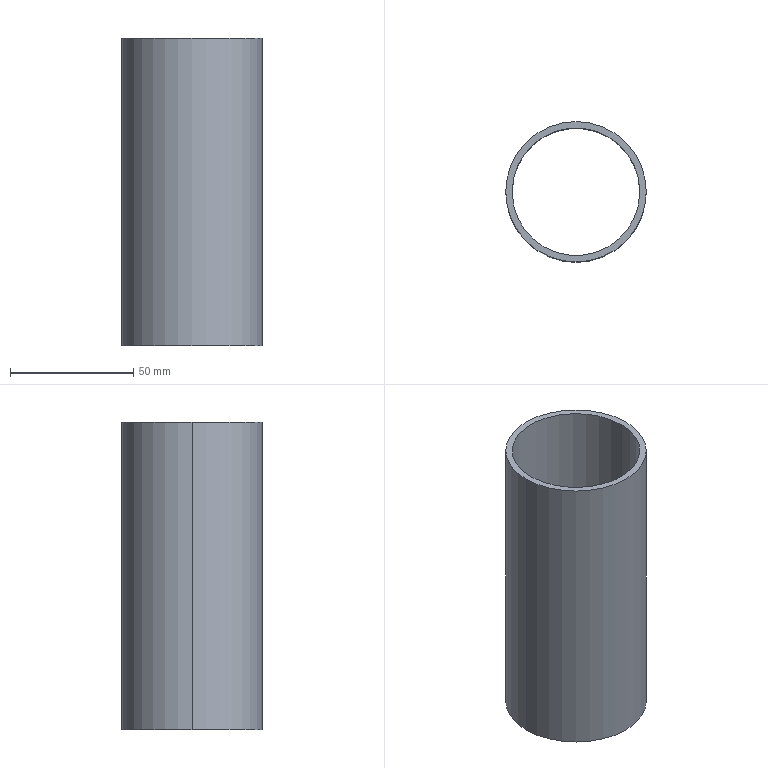Part | SolidWorks | features ExtruThin 1 | 1 solid | 6 faces | box 57 x 57 x 124.7 mm | volume 55410 mm3 | cylinder 4 | plane 2 | commonest cylinder face diameters 51.8 x2 57 x2
STEP:
#1=CARTESIAN_POINT('',(-25.9,0.,124.7));
#2=VERTEX_POINT('',#1);
#3=CARTESIAN_POINT('',(25.9,0.,124.7));
#4=VERTEX_POINT('',#3);
#5=CARTESIAN_POINT('',(0.,0.,124.7));
#6=DIRECTION('',(0.,0.,1.));
#7=DIRECTION('',(1.,0.,0.));
#8=AXIS2_PLACEMENT_3D('',#5,#6,#7);
#9=CIRCLE('',#8,25.9);
#10=EDGE_CURVE('',#2,#4,#9,.T.);
#11=ORIENTED_EDGE('',*,*,#10,.T.);
#12=CARTESIAN_POINT('',(25.9,0.,0.));
#13=VERTEX_POINT('',#12);
#14=CARTESIAN_POINT('',(25.9,0.,124.7));
#15=DIRECTION('',(0.,0.,-1.));
#16=VECTOR('',#15,1000.);
#17=LINE('',#14,#16);
#18=EDGE_CURVE('',#4,#13,#17,.T.);
#19=ORIENTED_EDGE('',*,*,#18,.T.);
#20=CARTESIAN_POINT('',(-25.9,0.,0.));
#21=VERTEX_POINT('',#20);
#22=CARTESIAN_POINT('',(0.,0.,0.));
#23=DIRECTION('',(0.,0.,1.));
#24=DIRECTION('',(1.,0.,0.));
#25=AXIS2_PLACEMENT_3D('',#22,#23,#24);
#26=CIRCLE('',#25,25.9);
#27=EDGE_CURVE('',#21,#13,#26,.T.);
#28=ORIENTED_EDGE('',*,*,#27,.F.);
#29=CARTESIAN_POINT('',(-25.9,0.,124.7));
#30=DIRECTION('',(0.,0.,-1.));
#31=VECTOR('',#30,1000.);
#32=LINE('',#29,#31);
#33=EDGE_CURVE('',#2,#21,#32,.T.);
#34=ORIENTED_EDGE('',*,*,#33,.F.);
#35=EDGE_LOOP('',(#11,#19,#28,#34));
#36=FACE_OUTER_BOUND('',#35,.T.);
#37=CARTESIAN_POINT('',(0.,0.,124.7));
#38=DIRECTION('',(0.,0.,-1.));
#39=DIRECTION('',(-1.,0.,0.));
#40=AXIS2_PLACEMENT_3D('',#37,#38,#39);
#41=CYLINDRICAL_SURFACE('',#40,25.9);
#42=ADVANCED_FACE('',(#36),#41,.F.);
#43=CARTESIAN_POINT('',(28.5,0.,124.7));
#44=VERTEX_POINT('',#43);
#45=CARTESIAN_POINT('',(-28.5,0.,124.7));
#46=VERTEX_POINT('',#45);
#47=CARTESIAN_POINT('',(0.,0.,124.7));
#48=DIRECTION('',(0.,0.,1.));
#49=DIRECTION('',(1.,0.,0.));
#50=AXIS2_PLACEMENT_3D('',#47,#48,#49);
#51=CIRCLE('',#50,28.5);
#52=EDGE_CURVE('',#44,#46,#51,.T.);
#53=ORIENTED_EDGE('',*,*,#52,.F.);
#54=CARTESIAN_POINT('',(28.5,0.,0.));
#55=VERTEX_POINT('',#54);
#56=CARTESIAN_POINT('',(28.5,0.,124.7));
#57=DIRECTION('',(0.,0.,-1.));
#58=VECTOR('',#57,1000.);
#59=LINE('',#56,#58);
#60=EDGE_CURVE('',#44,#55,#59,.T.);
#61=ORIENTED_EDGE('',*,*,#60,.T.);
#62=CARTESIAN_POINT('',(-28.5,0.,0.));
#63=VERTEX_POINT('',#62);
#64=CARTESIAN_POINT('',(0.,0.,0.));
#65=DIRECTION('',(0.,0.,1.));
#66=DIRECTION('',(1.,0.,0.));
#67=AXIS2_PLACEMENT_3D('',#64,#65,#66);
#68=CIRCLE('',#67,28.5);
#69=EDGE_CURVE('',#55,#63,#68,.T.);
#70=ORIENTED_EDGE('',*,*,#69,.T.);
#71=CARTESIAN_POINT('',(-28.5,0.,124.7));
#72=DIRECTION('',(0.,0.,-1.));
#73=VECTOR('',#72,1000.);
#74=LINE('',#71,#73);
#75=EDGE_CURVE('',#46,#63,#74,.T.);
#76=ORIENTED_EDGE('',*,*,#75,.F.);
#77=EDGE_LOOP('',(#53,#61,#70,#76));
#78=FACE_OUTER_BOUND('',#77,.T.);
#79=CARTESIAN_POINT('',(0.,0.,124.7));
#80=DIRECTION('',(0.,0.,-1.));
#81=DIRECTION('',(-1.,0.,0.));
#82=AXIS2_PLACEMENT_3D('',#79,#80,#81);
#83=CYLINDRICAL_SURFACE('',#82,28.5);
#84=ADVANCED_FACE('',(#78),#83,.T.);
#85=CARTESIAN_POINT('',(0.,0.,124.7));
#86=DIRECTION('',(0.,0.,1.));
#87=DIRECTION('',(1.,0.,0.));
#88=AXIS2_PLACEMENT_3D('',#85,#86,#87);
#89=CIRCLE('',#88,28.5);
#90=EDGE_CURVE('',#46,#44,#89,.T.);
#91=ORIENTED_EDGE('',*,*,#90,.T.);
#92=ORIENTED_EDGE('',*,*,#52,.T.);
#93=EDGE_LOOP('',(#91,#92));
#94=FACE_OUTER_BOUND('',#93,.T.);
#95=ORIENTED_EDGE('',*,*,#10,.F.);
#96=CARTESIAN_POINT('',(0.,0.,124.7));
#97=DIRECTION('',(0.,0.,1.));
#98=DIRECTION('',(1.,0.,0.));
#99=AXIS2_PLACEMENT_3D('',#96,#97,#98);
#100=CIRCLE('',#99,25.9);
#101=EDGE_CURVE('',#4,#2,#100,.T.);
#102=ORIENTED_EDGE('',*,*,#101,.F.);
#103=EDGE_LOOP('',(#95,#102));
#104=FACE_BOUND('',#103,.T.);
#105=CARTESIAN_POINT('',(0.,0.,124.7));
#106=DIRECTION('',(0.,0.,1.));
#107=DIRECTION('',(1.,0.,0.));
#108=AXIS2_PLACEMENT_3D('',#105,#106,#107);
#109=PLANE('',#108);
#110=ADVANCED_FACE('',(#94,#104),#109,.T.);
#111=CARTESIAN_POINT('',(0.,0.,0.));
#112=DIRECTION('',(0.,0.,1.));
#113=DIRECTION('',(1.,0.,0.));
#114=AXIS2_PLACEMENT_3D('',#111,#112,#113);
#115=CIRCLE('',#114,28.5);
#116=EDGE_CURVE('',#63,#55,#115,.T.);
#117=ORIENTED_EDGE('',*,*,#116,.F.);
#118=ORIENTED_EDGE('',*,*,#69,.F.);
#119=EDGE_LOOP('',(#117,#118));
#120=FACE_OUTER_BOUND('',#119,.T.);
#121=ORIENTED_EDGE('',*,*,#27,.T.);
#122=CARTESIAN_POINT('',(0.,0.,0.));
#123=DIRECTION('',(0.,0.,1.));
#124=DIRECTION('',(1.,0.,0.));
#125=AXIS2_PLACEMENT_3D('',#122,#123,#124);
#126=CIRCLE('',#125,25.9);
#127=EDGE_CURVE('',#13,#21,#126,.T.);
#128=ORIENTED_EDGE('',*,*,#127,.T.);
#129=EDGE_LOOP('',(#121,#128));
#130=FACE_BOUND('',#129,.T.);
#131=CARTESIAN_POINT('',(0.,0.,0.));
#132=DIRECTION('',(0.,0.,1.));
#133=DIRECTION('',(1.,0.,0.));
#134=AXIS2_PLACEMENT_3D('',#131,#132,#133);
#135=PLANE('',#134);
#136=ADVANCED_FACE('',(#120,#130),#135,.F.);
#137=ORIENTED_EDGE('',*,*,#60,.F.);
#138=ORIENTED_EDGE('',*,*,#90,.F.);
#139=ORIENTED_EDGE('',*,*,#75,.T.);
#140=ORIENTED_EDGE('',*,*,#116,.T.);
#141=EDGE_LOOP('',(#137,#138,#139,#140));
#142=FACE_OUTER_BOUND('',#141,.T.);
#143=CARTESIAN_POINT('',(0.,0.,124.7));
#144=DIRECTION('',(0.,0.,-1.));
#145=DIRECTION('',(-1.,0.,0.));
#146=AXIS2_PLACEMENT_3D('',#143,#144,#145);
#147=CYLINDRICAL_SURFACE('',#146,28.5);
#148=ADVANCED_FACE('',(#142),#147,.T.);
#149=ORIENTED_EDGE('',*,*,#18,.F.);
#150=ORIENTED_EDGE('',*,*,#101,.T.);
#151=ORIENTED_EDGE('',*,*,#33,.T.);
#152=ORIENTED_EDGE('',*,*,#127,.F.);
#153=EDGE_LOOP('',(#149,#150,#151,#152));
#154=FACE_OUTER_BOUND('',#153,.T.);
#155=CARTESIAN_POINT('',(0.,0.,124.7));
#156=DIRECTION('',(0.,0.,-1.));
#157=DIRECTION('',(-1.,0.,0.));
#158=AXIS2_PLACEMENT_3D('',#155,#156,#157);
#159=CYLINDRICAL_SURFACE('',#158,25.9);
#160=ADVANCED_FACE('',(#154),#159,.F.);
#161=CLOSED_SHELL('',(#42,#84,#110,#136,#148,#160));
#162=MANIFOLD_SOLID_BREP('',#161);
#163=CARTESIAN_POINT('',(0.,0.,0.));
#164=DIRECTION('',(0.,0.,1.));
#165=DIRECTION('',(1.,0.,0.));
#166=AXIS2_PLACEMENT_3D('',#163,#164,#165);
#167=(LENGTH_UNIT()NAMED_UNIT(*)SI_UNIT(.MILLI.,.METRE.));
#168=UNCERTAINTY_MEASURE_WITH_UNIT(LENGTH_MEASURE(0.00001),#167,'','');
#169=(NAMED_UNIT(*)PLANE_ANGLE_UNIT()SI_UNIT($,.RADIAN.));
#170=(NAMED_UNIT(*)SI_UNIT($,.STERADIAN.)SOLID_ANGLE_UNIT());
#171=(GEOMETRIC_REPRESENTATION_CONTEXT(3)GLOBAL_UNCERTAINTY_ASSIGNED_CONTEXT((#168))GLOBAL_UNIT_ASSIGNED_CONTEXT((#167,#169,#170))REPRESENTATION_CONTEXT('',''));
#172=ADVANCED_BREP_SHAPE_REPRESENTATION('',(#162,#166),#171);